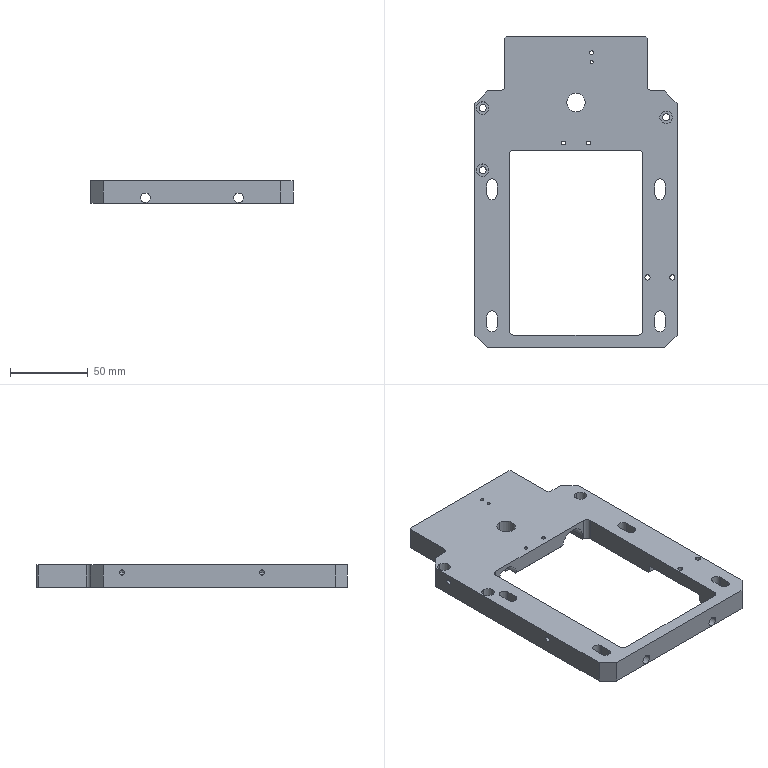Part | 1 solid | 149 faces | box 130 x 200 x 14.5 mm | volume 163035 mm3 | cylinder 78 | plane 60 | cone 11 | commonest cylinder face diameters 3.3 x12 6.5 x12 11 x12 2.5 x10 4.5 x6 6 x6